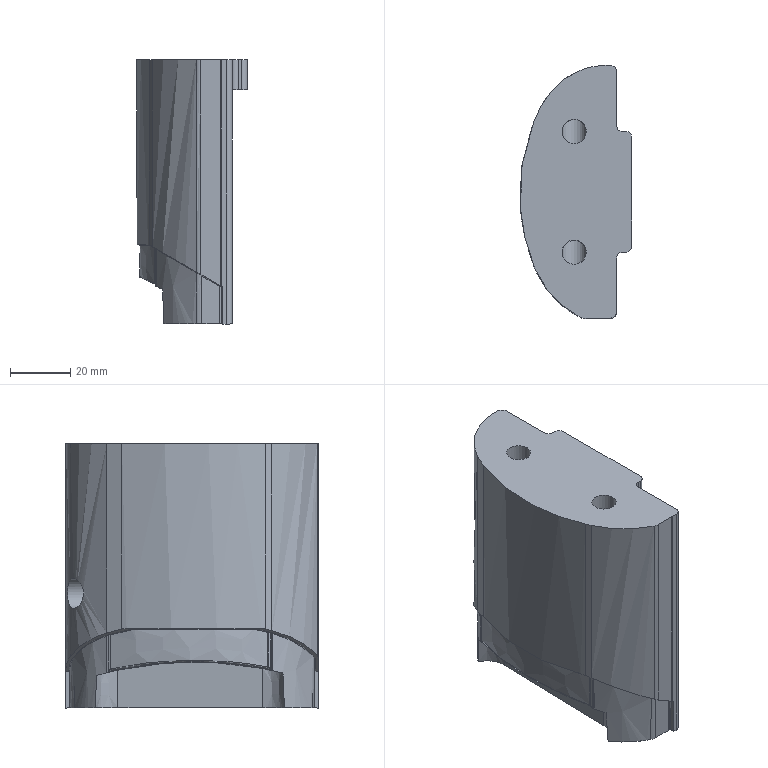Part | STEP file | solid 32 | 1 solid | 119 faces | box 37 x 83.675 x 87.541 mm | volume 174258 mm3 | spline 61 | plane 25 | cylinder 20 | cone 5 | sphere 4 | other 4 | commonest cylinder face diameters 4 x6 0.502 x4 0.603 x3 8 x3 2.01 x2 10 x1